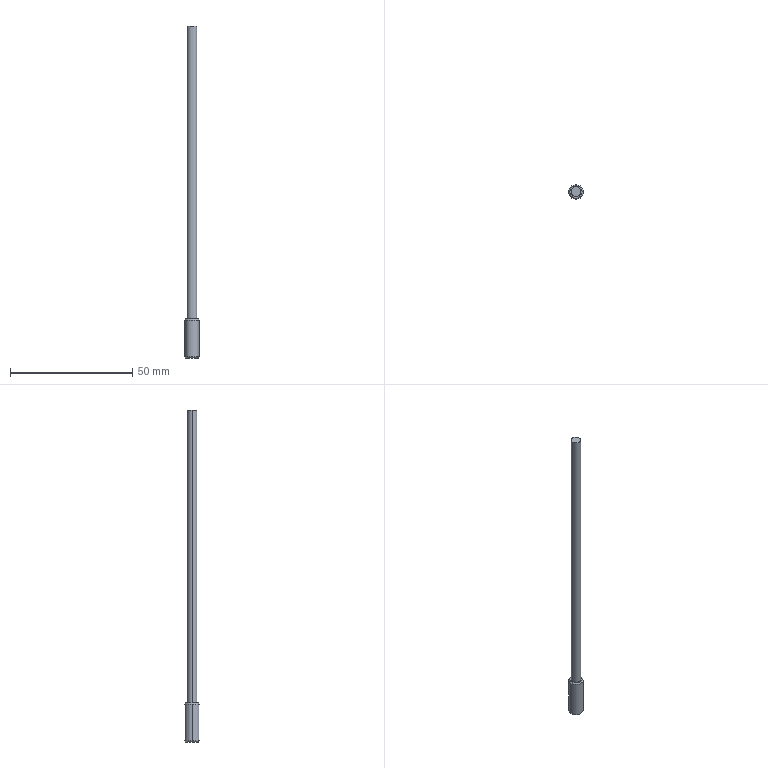Part | Creo | features DATUM PLANE 3, CURVE 2, PROTRUSION 2, CHAMFER 1, COORDINATE SYSTEM 1 | 1 solid | 11 faces | box 6 x 6 x 136 mm | volume 1956 mm3 | cone 4 | cylinder 4 | plane 3 | commonest cylinder face diameters 4 x2 6 x2
STEP:
#1=CARTESIAN_POINT('',(0.,0.,0.));
#2=DIRECTION('',(0.,0.,1.));
#3=DIRECTION('',(1.,0.,0.));
#4=AXIS2_PLACEMENT_3D('',#1,#2,#3);
#5=CARTESIAN_POINT('',(2.5,0.,0.));
#6=VERTEX_POINT('',#5);
#7=CARTESIAN_POINT('',(-2.5,0.,0.));
#8=VERTEX_POINT('',#7);
#9=CARTESIAN_POINT('',(0.,0.,0.));
#10=DIRECTION('',(0.,0.,-1.));
#11=DIRECTION('',(1.,0.,0.));
#12=AXIS2_PLACEMENT_3D('',#9,#10,#11);
#13=CIRCLE('',#12,2.5);
#14=EDGE_CURVE('',#6,#8,#13,.T.);
#15=ORIENTED_EDGE('',*,*,#14,.F.);
#16=CARTESIAN_POINT('',(0.,0.,0.));
#17=DIRECTION('',(0.,0.,-1.));
#18=DIRECTION('',(-1.,0.,0.));
#19=AXIS2_PLACEMENT_3D('',#16,#17,#18);
#20=CIRCLE('',#19,2.5);
#21=EDGE_CURVE('',#8,#6,#20,.T.);
#22=ORIENTED_EDGE('',*,*,#21,.F.);
#23=EDGE_LOOP('',(#15,#22));
#24=FACE_OUTER_BOUND('',#23,.F.);
#25=CARTESIAN_POINT('',(0.,0.,0.));
#26=DIRECTION('',(0.,0.,1.));
#27=DIRECTION('',(1.,0.,0.));
#28=AXIS2_PLACEMENT_3D('',#25,#26,#27);
#29=PLANE('',#28);
#30=ADVANCED_FACE('',(#24),#29,.F.);
#31=ORIENTED_EDGE('',*,*,#14,.T.);
#32=CARTESIAN_POINT('',(-3.,0.,0.5));
#33=VERTEX_POINT('',#32);
#34=CARTESIAN_POINT('',(-2.5,0.000000045,-0.000000008));
#35=DIRECTION('',(-0.7071,-0.000000006,0.7071));
#36=VECTOR('',#35,0.7071);
#37=LINE('',#34,#36);
#38=EDGE_CURVE('',#8,#33,#37,.T.);
#39=ORIENTED_EDGE('',*,*,#38,.T.);
#40=CARTESIAN_POINT('',(3.,0.,0.5));
#41=VERTEX_POINT('',#40);
#42=CARTESIAN_POINT('',(0.,0.,0.5));
#43=DIRECTION('',(0.,0.,-1.));
#44=DIRECTION('',(1.,0.,0.));
#45=AXIS2_PLACEMENT_3D('',#42,#43,#44);
#46=CIRCLE('',#45,3.);
#47=EDGE_CURVE('',#41,#33,#46,.T.);
#48=ORIENTED_EDGE('',*,*,#47,.F.);
#49=CARTESIAN_POINT('',(2.5,-0.000000045,-0.000000008));
#50=DIRECTION('',(0.7071,0.000000006,0.7071));
#51=VECTOR('',#50,0.7071);
#52=LINE('',#49,#51);
#53=EDGE_CURVE('',#6,#41,#52,.T.);
#54=ORIENTED_EDGE('',*,*,#53,.F.);
#55=EDGE_LOOP('',(#31,#39,#48,#54));
#56=FACE_OUTER_BOUND('',#55,.F.);
#57=CARTESIAN_POINT('',(0.,0.,0.25));
#58=DIRECTION('',(0.,0.,1.));
#59=DIRECTION('',(0.,-1.,0.));
#60=AXIS2_PLACEMENT_3D('',#57,#58,#59);
#61=CONICAL_SURFACE('',#60,2.75,45.);
#62=ADVANCED_FACE('',(#56),#61,.T.);
#63=ORIENTED_EDGE('',*,*,#21,.T.);
#64=ORIENTED_EDGE('',*,*,#53,.T.);
#65=CARTESIAN_POINT('',(0.,0.,0.5));
#66=DIRECTION('',(0.,0.,-1.));
#67=DIRECTION('',(-1.,0.,0.));
#68=AXIS2_PLACEMENT_3D('',#65,#66,#67);
#69=CIRCLE('',#68,3.);
#70=EDGE_CURVE('',#33,#41,#69,.T.);
#71=ORIENTED_EDGE('',*,*,#70,.F.);
#72=ORIENTED_EDGE('',*,*,#38,.F.);
#73=EDGE_LOOP('',(#63,#64,#71,#72));
#74=FACE_OUTER_BOUND('',#73,.F.);
#75=CARTESIAN_POINT('',(0.,0.,0.25));
#76=DIRECTION('',(0.,0.,1.));
#77=DIRECTION('',(0.,-1.,0.));
#78=AXIS2_PLACEMENT_3D('',#75,#76,#77);
#79=CONICAL_SURFACE('',#78,2.75,45.);
#80=ADVANCED_FACE('',(#74),#79,.T.);
#81=ORIENTED_EDGE('',*,*,#70,.T.);
#82=CARTESIAN_POINT('',(3.,0.,15.5));
#83=VERTEX_POINT('',#82);
#84=CARTESIAN_POINT('',(3.,-0.000000041,0.5));
#85=DIRECTION('',(0.,0.,1.));
#86=VECTOR('',#85,15.);
#87=LINE('',#84,#86);
#88=EDGE_CURVE('',#41,#83,#87,.T.);
#89=ORIENTED_EDGE('',*,*,#88,.T.);
#90=CARTESIAN_POINT('',(-3.,0.,15.5));
#91=VERTEX_POINT('',#90);
#92=CARTESIAN_POINT('',(0.,0.,15.5));
#93=DIRECTION('',(0.,0.,1.));
#94=DIRECTION('',(1.,0.,0.));
#95=AXIS2_PLACEMENT_3D('',#92,#93,#94);
#96=CIRCLE('',#95,3.);
#97=EDGE_CURVE('',#83,#91,#96,.T.);
#98=ORIENTED_EDGE('',*,*,#97,.T.);
#99=CARTESIAN_POINT('',(-3.,0.000000041,0.5));
#100=DIRECTION('',(0.,0.,1.));
#101=VECTOR('',#100,15.);
#102=LINE('',#99,#101);
#103=EDGE_CURVE('',#33,#91,#102,.T.);
#104=ORIENTED_EDGE('',*,*,#103,.F.);
#105=EDGE_LOOP('',(#81,#89,#98,#104));
#106=FACE_OUTER_BOUND('',#105,.F.);
#107=CARTESIAN_POINT('',(0.,0.,0.));
#108=DIRECTION('',(0.,0.,1.));
#109=DIRECTION('',(1.,0.,0.));
#110=AXIS2_PLACEMENT_3D('',#107,#108,#109);
#111=CYLINDRICAL_SURFACE('',#110,3.);
#112=ADVANCED_FACE('',(#106),#111,.T.);
#113=ORIENTED_EDGE('',*,*,#47,.T.);
#114=ORIENTED_EDGE('',*,*,#103,.T.);
#115=CARTESIAN_POINT('',(0.,0.,15.5));
#116=DIRECTION('',(0.,0.,1.));
#117=DIRECTION('',(-1.,0.,0.));
#118=AXIS2_PLACEMENT_3D('',#115,#116,#117);
#119=CIRCLE('',#118,3.);
#120=EDGE_CURVE('',#91,#83,#119,.T.);
#121=ORIENTED_EDGE('',*,*,#120,.T.);
#122=ORIENTED_EDGE('',*,*,#88,.F.);
#123=EDGE_LOOP('',(#113,#114,#121,#122));
#124=FACE_OUTER_BOUND('',#123,.F.);
#125=CARTESIAN_POINT('',(0.,0.,0.));
#126=DIRECTION('',(0.,0.,1.));
#127=DIRECTION('',(1.,0.,0.));
#128=AXIS2_PLACEMENT_3D('',#125,#126,#127);
#129=CYLINDRICAL_SURFACE('',#128,3.);
#130=ADVANCED_FACE('',(#124),#129,.T.);
#131=CARTESIAN_POINT('',(-2.5,0.,16.));
#132=VERTEX_POINT('',#131);
#133=CARTESIAN_POINT('',(2.5,0.,16.));
#134=VERTEX_POINT('',#133);
#135=CARTESIAN_POINT('',(0.,0.,16.));
#136=DIRECTION('',(0.,0.,1.));
#137=DIRECTION('',(-1.,0.,0.));
#138=AXIS2_PLACEMENT_3D('',#135,#136,#137);
#139=CIRCLE('',#138,2.5);
#140=EDGE_CURVE('',#132,#134,#139,.T.);
#141=ORIENTED_EDGE('',*,*,#140,.T.);
#142=CARTESIAN_POINT('',(2.5,-0.000000045,16.));
#143=DIRECTION('',(0.7071,0.000000006,-0.7071));
#144=VECTOR('',#143,0.7071);
#145=LINE('',#142,#144);
#146=EDGE_CURVE('',#134,#83,#145,.T.);
#147=ORIENTED_EDGE('',*,*,#146,.T.);
#148=ORIENTED_EDGE('',*,*,#120,.F.);
#149=CARTESIAN_POINT('',(-2.5,0.000000045,16.));
#150=DIRECTION('',(-0.7071,-0.000000006,-0.7071));
#151=VECTOR('',#150,0.7071);
#152=LINE('',#149,#151);
#153=EDGE_CURVE('',#132,#91,#152,.T.);
#154=ORIENTED_EDGE('',*,*,#153,.F.);
#155=EDGE_LOOP('',(#141,#147,#148,#154));
#156=FACE_OUTER_BOUND('',#155,.F.);
#157=CARTESIAN_POINT('',(0.,0.,15.75));
#158=DIRECTION('',(0.,0.,-1.));
#159=DIRECTION('',(0.,-1.,0.));
#160=AXIS2_PLACEMENT_3D('',#157,#158,#159);
#161=CONICAL_SURFACE('',#160,2.75,45.);
#162=ADVANCED_FACE('',(#156),#161,.T.);
#163=ORIENTED_EDGE('',*,*,#140,.F.);
#164=CARTESIAN_POINT('',(0.,0.,16.));
#165=DIRECTION('',(0.,0.,1.));
#166=DIRECTION('',(1.,0.,0.));
#167=AXIS2_PLACEMENT_3D('',#164,#165,#166);
#168=CIRCLE('',#167,2.5);
#169=EDGE_CURVE('',#134,#132,#168,.T.);
#170=ORIENTED_EDGE('',*,*,#169,.F.);
#171=EDGE_LOOP('',(#163,#170));
#172=FACE_OUTER_BOUND('',#171,.F.);
#173=CARTESIAN_POINT('',(2.,0.,16.));
#174=VERTEX_POINT('',#173);
#175=CARTESIAN_POINT('',(-2.,0.,16.));
#176=VERTEX_POINT('',#175);
#177=CARTESIAN_POINT('',(0.,0.,16.));
#178=DIRECTION('',(0.,0.,1.));
#179=DIRECTION('',(1.,0.,0.));
#180=AXIS2_PLACEMENT_3D('',#177,#178,#179);
#181=CIRCLE('',#180,2.);
#182=EDGE_CURVE('',#174,#176,#181,.T.);
#183=ORIENTED_EDGE('',*,*,#182,.T.);
#184=CARTESIAN_POINT('',(0.,0.,16.));
#185=DIRECTION('',(0.,0.,1.));
#186=DIRECTION('',(-1.,0.,0.));
#187=AXIS2_PLACEMENT_3D('',#184,#185,#186);
#188=CIRCLE('',#187,2.);
#189=EDGE_CURVE('',#176,#174,#188,.T.);
#190=ORIENTED_EDGE('',*,*,#189,.T.);
#191=EDGE_LOOP('',(#183,#190));
#192=FACE_BOUND('',#191,.F.);
#193=CARTESIAN_POINT('',(0.,0.,16.));
#194=DIRECTION('',(0.,0.,1.));
#195=DIRECTION('',(1.,0.,0.));
#196=AXIS2_PLACEMENT_3D('',#193,#194,#195);
#197=PLANE('',#196);
#198=ADVANCED_FACE('',(#172,#192),#197,.T.);
#199=ORIENTED_EDGE('',*,*,#182,.F.);
#200=CARTESIAN_POINT('',(2.,0.,136.));
#201=VERTEX_POINT('',#200);
#202=CARTESIAN_POINT('',(2.,0.,16.));
#203=DIRECTION('',(0.,0.,1.));
#204=VECTOR('',#203,120.);
#205=LINE('',#202,#204);
#206=EDGE_CURVE('',#174,#201,#205,.T.);
#207=ORIENTED_EDGE('',*,*,#206,.T.);
#208=CARTESIAN_POINT('',(-2.,0.,136.));
#209=VERTEX_POINT('',#208);
#210=CARTESIAN_POINT('',(0.,0.,136.));
#211=DIRECTION('',(0.,0.,1.));
#212=DIRECTION('',(1.,0.,0.));
#213=AXIS2_PLACEMENT_3D('',#210,#211,#212);
#214=CIRCLE('',#213,2.);
#215=EDGE_CURVE('',#201,#209,#214,.T.);
#216=ORIENTED_EDGE('',*,*,#215,.T.);
#217=CARTESIAN_POINT('',(-2.,0.,16.));
#218=DIRECTION('',(0.,0.,1.));
#219=VECTOR('',#218,120.);
#220=LINE('',#217,#219);
#221=EDGE_CURVE('',#176,#209,#220,.T.);
#222=ORIENTED_EDGE('',*,*,#221,.F.);
#223=EDGE_LOOP('',(#199,#207,#216,#222));
#224=FACE_OUTER_BOUND('',#223,.F.);
#225=CARTESIAN_POINT('',(0.,0.,16.));
#226=DIRECTION('',(0.,0.,1.));
#227=DIRECTION('',(1.,0.,0.));
#228=AXIS2_PLACEMENT_3D('',#225,#226,#227);
#229=CYLINDRICAL_SURFACE('',#228,2.);
#230=ADVANCED_FACE('',(#224),#229,.T.);
#231=ORIENTED_EDGE('',*,*,#189,.F.);
#232=ORIENTED_EDGE('',*,*,#221,.T.);
#233=CARTESIAN_POINT('',(0.,0.,136.));
#234=DIRECTION('',(0.,0.,1.));
#235=DIRECTION('',(-1.,0.,0.));
#236=AXIS2_PLACEMENT_3D('',#233,#234,#235);
#237=CIRCLE('',#236,2.);
#238=EDGE_CURVE('',#209,#201,#237,.T.);
#239=ORIENTED_EDGE('',*,*,#238,.T.);
#240=ORIENTED_EDGE('',*,*,#206,.F.);
#241=EDGE_LOOP('',(#231,#232,#239,#240));
#242=FACE_OUTER_BOUND('',#241,.F.);
#243=CARTESIAN_POINT('',(0.,0.,16.));
#244=DIRECTION('',(0.,0.,1.));
#245=DIRECTION('',(1.,0.,0.));
#246=AXIS2_PLACEMENT_3D('',#243,#244,#245);
#247=CYLINDRICAL_SURFACE('',#246,2.);
#248=ADVANCED_FACE('',(#242),#247,.T.);
#249=ORIENTED_EDGE('',*,*,#215,.F.);
#250=ORIENTED_EDGE('',*,*,#238,.F.);
#251=EDGE_LOOP('',(#249,#250));
#252=FACE_OUTER_BOUND('',#251,.F.);
#253=CARTESIAN_POINT('',(0.,0.,136.));
#254=DIRECTION('',(0.,0.,1.));
#255=DIRECTION('',(1.,0.,0.));
#256=AXIS2_PLACEMENT_3D('',#253,#254,#255);
#257=PLANE('',#256);
#258=ADVANCED_FACE('',(#252),#257,.T.);
#259=ORIENTED_EDGE('',*,*,#169,.T.);
#260=ORIENTED_EDGE('',*,*,#153,.T.);
#261=ORIENTED_EDGE('',*,*,#97,.F.);
#262=ORIENTED_EDGE('',*,*,#146,.F.);
#263=EDGE_LOOP('',(#259,#260,#261,#262));
#264=FACE_OUTER_BOUND('',#263,.F.);
#265=CARTESIAN_POINT('',(0.,0.,15.75));
#266=DIRECTION('',(0.,0.,-1.));
#267=DIRECTION('',(0.,-1.,0.));
#268=AXIS2_PLACEMENT_3D('',#265,#266,#267);
#269=CONICAL_SURFACE('',#268,2.75,45.);
#270=ADVANCED_FACE('',(#264),#269,.T.);
#271=CLOSED_SHELL('',(#30,#62,#80,#112,#130,#162,#198,#230,#248,#258,#270));
#272=MANIFOLD_SOLID_BREP('',#271);
#273=(LENGTH_UNIT()NAMED_UNIT(*)SI_UNIT(.MILLI.,.METRE.));
#274=UNCERTAINTY_MEASURE_WITH_UNIT(LENGTH_MEASURE(0.01363),#273,'','');
#275=(NAMED_UNIT(*)PLANE_ANGLE_UNIT()SI_UNIT($,.RADIAN.));
#276=PLANE_ANGLE_MEASURE_WITH_UNIT(PLANE_ANGLE_MEASURE(0.01745),#275);
#277=(CONVERSION_BASED_UNIT('DEGREE',#276)NAMED_UNIT(*)PLANE_ANGLE_UNIT());
#278=(NAMED_UNIT(*)SI_UNIT($,.STERADIAN.)SOLID_ANGLE_UNIT());
#279=(GEOMETRIC_REPRESENTATION_CONTEXT(3)GLOBAL_UNCERTAINTY_ASSIGNED_CONTEXT((#274))GLOBAL_UNIT_ASSIGNED_CONTEXT((#273,#277,#278))REPRESENTATION_CONTEXT('',''));
#280=ADVANCED_BREP_SHAPE_REPRESENTATION('',(#4,#272),#279);